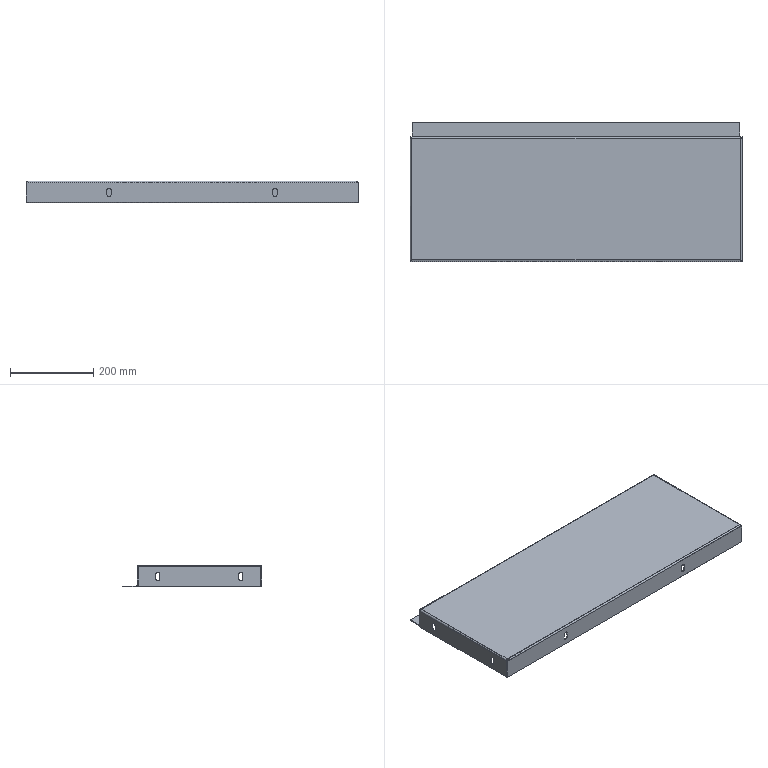Part | STEP file | SYL_0392D6J1SYL0380DJ1006_2_11- | 1 solid | 90 faces | box 800 x 335 x 53 mm | volume 743196 mm3 | plane 48 | cylinder 34 | spline 8 | commonest cylinder face diameters 10 x24 4 x5 8 x5